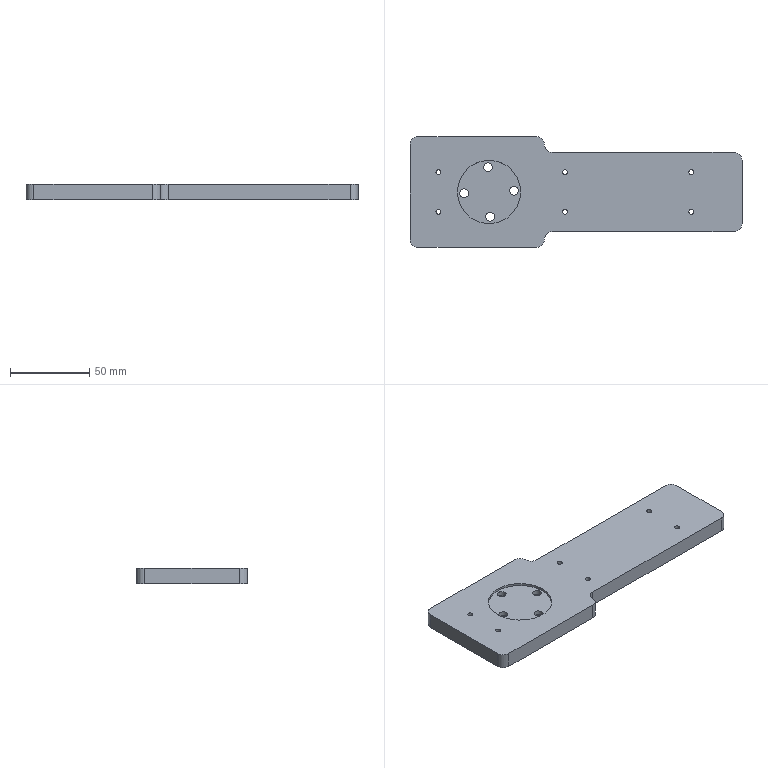Part | STEP file | SynoNew-0304-038 | 1 solid | 38 faces | box 210 x 70 x 10 mm | volume 117309 mm3 | cylinder 24 | plane 14 | commonest cylinder face diameters 10 x12 3.2 x6 5.5 x4 4 x1 40.02 x1
STEP:
#1=CARTESIAN_POINT('',(51.,0.,0.));
#2=VERTEX_POINT('',#1);
#3=CARTESIAN_POINT('',(55.,0.,0.));
#4=VERTEX_POINT('',#3);
#5=CARTESIAN_POINT('',(53.,0.,0.));
#6=DIRECTION('',(0.,0.,1.));
#7=DIRECTION('',(-1.,0.,0.));
#8=AXIS2_PLACEMENT_3D('',#5,#6,#7);
#9=CIRCLE('',#8,2.);
#10=EDGE_CURVE('',#2,#4,#9,.T.);
#11=ORIENTED_EDGE('',*,*,#10,.F.);
#12=CARTESIAN_POINT('',(53.,0.,0.));
#13=DIRECTION('',(0.,0.,1.));
#14=DIRECTION('',(-1.,0.,0.));
#15=AXIS2_PLACEMENT_3D('',#12,#13,#14);
#16=CIRCLE('',#15,2.);
#17=EDGE_CURVE('',#4,#2,#16,.T.);
#18=ORIENTED_EDGE('',*,*,#17,.F.);
#19=CARTESIAN_POINT('',(55.,0.,4.));
#20=VERTEX_POINT('',#19);
#21=CARTESIAN_POINT('',(55.,0.,0.));
#22=DIRECTION('',(0.,0.,1.));
#23=VECTOR('',#22,2.);
#24=LINE('',#21,#23);
#25=EDGE_CURVE('',#4,#20,#24,.T.);
#26=ORIENTED_EDGE('',*,*,#25,.T.);
#27=CARTESIAN_POINT('',(51.,0.,4.));
#28=VERTEX_POINT('',#27);
#29=CARTESIAN_POINT('',(53.,0.,4.));
#30=DIRECTION('',(0.,0.,1.));
#31=DIRECTION('',(-1.,0.,0.));
#32=AXIS2_PLACEMENT_3D('',#29,#30,#31);
#33=CIRCLE('',#32,2.);
#34=EDGE_CURVE('',#20,#28,#33,.T.);
#35=ORIENTED_EDGE('',*,*,#34,.T.);
#36=CARTESIAN_POINT('',(53.,0.,4.));
#37=DIRECTION('',(0.,0.,1.));
#38=DIRECTION('',(-1.,0.,0.));
#39=AXIS2_PLACEMENT_3D('',#36,#37,#38);
#40=CIRCLE('',#39,2.);
#41=EDGE_CURVE('',#28,#20,#40,.T.);
#42=ORIENTED_EDGE('',*,*,#41,.T.);
#43=ORIENTED_EDGE('',*,*,#25,.F.);
#44=EDGE_LOOP('',(#11,#18,#26,#35,#42,#43));
#45=FACE_OUTER_BOUND('',#44,.T.);
#46=CARTESIAN_POINT('',(53.,0.,0.));
#47=DIRECTION('',(0.,0.,1.));
#48=DIRECTION('',(-1.,0.,0.));
#49=AXIS2_PLACEMENT_3D('',#46,#47,#48);
#50=CYLINDRICAL_SURFACE('',#49,2.);
#51=ADVANCED_FACE('',(#45),#50,.F.);
#52=ORIENTED_EDGE('',*,*,#41,.F.);
#53=ORIENTED_EDGE('',*,*,#34,.F.);
#54=EDGE_LOOP('',(#52,#53));
#55=FACE_OUTER_BOUND('',#54,.T.);
#56=CARTESIAN_POINT('',(53.,0.,4.));
#57=DIRECTION('',(0.,0.,-1.));
#58=DIRECTION('',(-1.,0.,0.));
#59=AXIS2_PLACEMENT_3D('',#56,#57,#58);
#60=PLANE('',#59);
#61=ADVANCED_FACE('',(#55),#60,.T.);
#62=CARTESIAN_POINT('',(-105.4,-12.5,10.));
#63=VERTEX_POINT('',#62);
#64=CARTESIAN_POINT('',(-108.6,-12.5,10.));
#65=VERTEX_POINT('',#64);
#66=CARTESIAN_POINT('',(-107.,-12.5,10.));
#67=DIRECTION('',(0.,0.,-1.));
#68=DIRECTION('',(1.,0.,0.));
#69=AXIS2_PLACEMENT_3D('',#66,#67,#68);
#70=CIRCLE('',#69,1.6);
#71=EDGE_CURVE('',#63,#65,#70,.T.);
#72=ORIENTED_EDGE('',*,*,#71,.F.);
#73=CARTESIAN_POINT('',(-107.,-12.5,10.));
#74=DIRECTION('',(0.,0.,-1.));
#75=DIRECTION('',(1.,0.,0.));
#76=AXIS2_PLACEMENT_3D('',#73,#74,#75);
#77=CIRCLE('',#76,1.6);
#78=EDGE_CURVE('',#65,#63,#77,.T.);
#79=ORIENTED_EDGE('',*,*,#78,.F.);
#80=CARTESIAN_POINT('',(-108.6,-12.5,0.));
#81=VERTEX_POINT('',#80);
#82=CARTESIAN_POINT('',(-108.6,-12.5,-211.585));
#83=DIRECTION('',(0.,0.,-1.));
#84=VECTOR('',#83,1.6);
#85=LINE('',#82,#84);
#86=EDGE_CURVE('',#65,#81,#85,.T.);
#87=ORIENTED_EDGE('',*,*,#86,.T.);
#88=CARTESIAN_POINT('',(-107.,-12.5,0.));
#89=DIRECTION('',(0.,0.,1.));
#90=DIRECTION('',(1.,0.,0.));
#91=AXIS2_PLACEMENT_3D('',#88,#89,#90);
#92=CIRCLE('',#91,1.6);
#93=EDGE_CURVE('',#81,#81,#92,.T.);
#94=ORIENTED_EDGE('',*,*,#93,.F.);
#95=ORIENTED_EDGE('',*,*,#86,.F.);
#96=EDGE_LOOP('',(#72,#79,#87,#94,#95));
#97=FACE_OUTER_BOUND('',#96,.T.);
#98=CARTESIAN_POINT('',(-107.,-12.5,-211.585));
#99=DIRECTION('',(0.,0.,1.));
#100=DIRECTION('',(1.,0.,0.));
#101=AXIS2_PLACEMENT_3D('',#98,#99,#100);
#102=CYLINDRICAL_SURFACE('',#101,1.6);
#103=ADVANCED_FACE('',(#97),#102,.F.);
#104=CARTESIAN_POINT('',(-25.4,-12.5,10.));
#105=VERTEX_POINT('',#104);
#106=CARTESIAN_POINT('',(-28.6,-12.5,10.));
#107=VERTEX_POINT('',#106);
#108=CARTESIAN_POINT('',(-27.,-12.5,10.));
#109=DIRECTION('',(0.,0.,-1.));
#110=DIRECTION('',(1.,0.,0.));
#111=AXIS2_PLACEMENT_3D('',#108,#109,#110);
#112=CIRCLE('',#111,1.6);
#113=EDGE_CURVE('',#105,#107,#112,.T.);
#114=ORIENTED_EDGE('',*,*,#113,.F.);
#115=CARTESIAN_POINT('',(-27.,-12.5,10.));
#116=DIRECTION('',(0.,0.,-1.));
#117=DIRECTION('',(1.,0.,0.));
#118=AXIS2_PLACEMENT_3D('',#115,#116,#117);
#119=CIRCLE('',#118,1.6);
#120=EDGE_CURVE('',#107,#105,#119,.T.);
#121=ORIENTED_EDGE('',*,*,#120,.F.);
#122=CARTESIAN_POINT('',(-28.6,-12.5,0.));
#123=VERTEX_POINT('',#122);
#124=CARTESIAN_POINT('',(-28.6,-12.5,-211.585));
#125=DIRECTION('',(0.,0.,-1.));
#126=VECTOR('',#125,1.6);
#127=LINE('',#124,#126);
#128=EDGE_CURVE('',#107,#123,#127,.T.);
#129=ORIENTED_EDGE('',*,*,#128,.T.);
#130=CARTESIAN_POINT('',(-27.,-12.5,0.));
#131=DIRECTION('',(0.,0.,1.));
#132=DIRECTION('',(1.,0.,0.));
#133=AXIS2_PLACEMENT_3D('',#130,#131,#132);
#134=CIRCLE('',#133,1.6);
#135=EDGE_CURVE('',#123,#123,#134,.T.);
#136=ORIENTED_EDGE('',*,*,#135,.F.);
#137=ORIENTED_EDGE('',*,*,#128,.F.);
#138=EDGE_LOOP('',(#114,#121,#129,#136,#137));
#139=FACE_OUTER_BOUND('',#138,.T.);
#140=CARTESIAN_POINT('',(-27.,-12.5,-211.585));
#141=DIRECTION('',(0.,0.,1.));
#142=DIRECTION('',(1.,0.,0.));
#143=AXIS2_PLACEMENT_3D('',#140,#141,#142);
#144=CYLINDRICAL_SURFACE('',#143,1.6);
#145=ADVANCED_FACE('',(#139),#144,.F.);
#146=CARTESIAN_POINT('',(54.6,12.5,10.));
#147=VERTEX_POINT('',#146);
#148=CARTESIAN_POINT('',(51.4,12.5,10.));
#149=VERTEX_POINT('',#148);
#150=CARTESIAN_POINT('',(53.,12.5,10.));
#151=DIRECTION('',(0.,0.,-1.));
#152=DIRECTION('',(1.,0.,0.));
#153=AXIS2_PLACEMENT_3D('',#150,#151,#152);
#154=CIRCLE('',#153,1.6);
#155=EDGE_CURVE('',#147,#149,#154,.T.);
#156=ORIENTED_EDGE('',*,*,#155,.F.);
#157=CARTESIAN_POINT('',(53.,12.5,10.));
#158=DIRECTION('',(0.,0.,-1.));
#159=DIRECTION('',(1.,0.,0.));
#160=AXIS2_PLACEMENT_3D('',#157,#158,#159);
#161=CIRCLE('',#160,1.6);
#162=EDGE_CURVE('',#149,#147,#161,.T.);
#163=ORIENTED_EDGE('',*,*,#162,.F.);
#164=CARTESIAN_POINT('',(51.4,12.5,0.));
#165=VERTEX_POINT('',#164);
#166=CARTESIAN_POINT('',(51.4,12.5,-211.585));
#167=DIRECTION('',(0.,0.,-1.));
#168=VECTOR('',#167,1.6);
#169=LINE('',#166,#168);
#170=EDGE_CURVE('',#149,#165,#169,.T.);
#171=ORIENTED_EDGE('',*,*,#170,.T.);
#172=CARTESIAN_POINT('',(53.,12.5,0.));
#173=DIRECTION('',(0.,0.,1.));
#174=DIRECTION('',(1.,0.,0.));
#175=AXIS2_PLACEMENT_3D('',#172,#173,#174);
#176=CIRCLE('',#175,1.6);
#177=EDGE_CURVE('',#165,#165,#176,.T.);
#178=ORIENTED_EDGE('',*,*,#177,.F.);
#179=ORIENTED_EDGE('',*,*,#170,.F.);
#180=EDGE_LOOP('',(#156,#163,#171,#178,#179));
#181=FACE_OUTER_BOUND('',#180,.T.);
#182=CARTESIAN_POINT('',(53.,12.5,-211.585));
#183=DIRECTION('',(0.,0.,1.));
#184=DIRECTION('',(1.,0.,0.));
#185=AXIS2_PLACEMENT_3D('',#182,#183,#184);
#186=CYLINDRICAL_SURFACE('',#185,1.6);
#187=ADVANCED_FACE('',(#181),#186,.F.);
#188=CARTESIAN_POINT('',(54.6,-12.5,10.));
#189=VERTEX_POINT('',#188);
#190=CARTESIAN_POINT('',(51.4,-12.5,10.));
#191=VERTEX_POINT('',#190);
#192=CARTESIAN_POINT('',(53.,-12.5,10.));
#193=DIRECTION('',(0.,0.,-1.));
#194=DIRECTION('',(1.,0.,0.));
#195=AXIS2_PLACEMENT_3D('',#192,#193,#194);
#196=CIRCLE('',#195,1.6);
#197=EDGE_CURVE('',#189,#191,#196,.T.);
#198=ORIENTED_EDGE('',*,*,#197,.F.);
#199=CARTESIAN_POINT('',(53.,-12.5,10.));
#200=DIRECTION('',(0.,0.,-1.));
#201=DIRECTION('',(1.,0.,0.));
#202=AXIS2_PLACEMENT_3D('',#199,#200,#201);
#203=CIRCLE('',#202,1.6);
#204=EDGE_CURVE('',#191,#189,#203,.T.);
#205=ORIENTED_EDGE('',*,*,#204,.F.);
#206=CARTESIAN_POINT('',(51.4,-12.5,0.));
#207=VERTEX_POINT('',#206);
#208=CARTESIAN_POINT('',(51.4,-12.5,-211.585));
#209=DIRECTION('',(0.,0.,-1.));
#210=VECTOR('',#209,1.6);
#211=LINE('',#208,#210);
#212=EDGE_CURVE('',#191,#207,#211,.T.);
#213=ORIENTED_EDGE('',*,*,#212,.T.);
#214=CARTESIAN_POINT('',(53.,-12.5,0.));
#215=DIRECTION('',(0.,0.,1.));
#216=DIRECTION('',(1.,0.,0.));
#217=AXIS2_PLACEMENT_3D('',#214,#215,#216);
#218=CIRCLE('',#217,1.6);
#219=EDGE_CURVE('',#207,#207,#218,.T.);
#220=ORIENTED_EDGE('',*,*,#219,.F.);
#221=ORIENTED_EDGE('',*,*,#212,.F.);
#222=EDGE_LOOP('',(#198,#205,#213,#220,#221));
#223=FACE_OUTER_BOUND('',#222,.T.);
#224=CARTESIAN_POINT('',(53.,-12.5,-211.585));
#225=DIRECTION('',(0.,0.,1.));
#226=DIRECTION('',(1.,0.,0.));
#227=AXIS2_PLACEMENT_3D('',#224,#225,#226);
#228=CYLINDRICAL_SURFACE('',#227,1.6);
#229=ADVANCED_FACE('',(#223),#228,.F.);
#230=CARTESIAN_POINT('',(-25.4,12.5,10.));
#231=VERTEX_POINT('',#230);
#232=CARTESIAN_POINT('',(-28.6,12.5,10.));
#233=VERTEX_POINT('',#232);
#234=CARTESIAN_POINT('',(-27.,12.5,10.));
#235=DIRECTION('',(0.,0.,-1.));
#236=DIRECTION('',(1.,0.,0.));
#237=AXIS2_PLACEMENT_3D('',#234,#235,#236);
#238=CIRCLE('',#237,1.6);
#239=EDGE_CURVE('',#231,#233,#238,.T.);
#240=ORIENTED_EDGE('',*,*,#239,.F.);
#241=CARTESIAN_POINT('',(-27.,12.5,10.));
#242=DIRECTION('',(0.,0.,-1.));
#243=DIRECTION('',(1.,0.,0.));
#244=AXIS2_PLACEMENT_3D('',#241,#242,#243);
#245=CIRCLE('',#244,1.6);
#246=EDGE_CURVE('',#233,#231,#245,.T.);
#247=ORIENTED_EDGE('',*,*,#246,.F.);
#248=CARTESIAN_POINT('',(-28.6,12.5,0.));
#249=VERTEX_POINT('',#248);
#250=CARTESIAN_POINT('',(-28.6,12.5,-211.585));
#251=DIRECTION('',(0.,0.,-1.));
#252=VECTOR('',#251,1.6);
#253=LINE('',#250,#252);
#254=EDGE_CURVE('',#233,#249,#253,.T.);
#255=ORIENTED_EDGE('',*,*,#254,.T.);
#256=CARTESIAN_POINT('',(-27.,12.5,0.));
#257=DIRECTION('',(0.,0.,1.));
#258=DIRECTION('',(1.,0.,0.));
#259=AXIS2_PLACEMENT_3D('',#256,#257,#258);
#260=CIRCLE('',#259,1.6);
#261=EDGE_CURVE('',#249,#249,#260,.T.);
#262=ORIENTED_EDGE('',*,*,#261,.F.);
#263=ORIENTED_EDGE('',*,*,#254,.F.);
#264=EDGE_LOOP('',(#240,#247,#255,#262,#263));
#265=FACE_OUTER_BOUND('',#264,.T.);
#266=CARTESIAN_POINT('',(-27.,12.5,-211.585));
#267=DIRECTION('',(0.,0.,1.));
#268=DIRECTION('',(1.,0.,0.));
#269=AXIS2_PLACEMENT_3D('',#266,#267,#268);
#270=CYLINDRICAL_SURFACE('',#269,1.6);
#271=ADVANCED_FACE('',(#265),#270,.F.);
#272=CARTESIAN_POINT('',(-105.4,12.5,10.));
#273=VERTEX_POINT('',#272);
#274=CARTESIAN_POINT('',(-108.6,12.5,10.));
#275=VERTEX_POINT('',#274);
#276=CARTESIAN_POINT('',(-107.,12.5,10.));
#277=DIRECTION('',(0.,0.,-1.));
#278=DIRECTION('',(1.,0.,0.));
#279=AXIS2_PLACEMENT_3D('',#276,#277,#278);
#280=CIRCLE('',#279,1.6);
#281=EDGE_CURVE('',#273,#275,#280,.T.);
#282=ORIENTED_EDGE('',*,*,#281,.F.);
#283=CARTESIAN_POINT('',(-107.,12.5,10.));
#284=DIRECTION('',(0.,0.,-1.));
#285=DIRECTION('',(1.,0.,0.));
#286=AXIS2_PLACEMENT_3D('',#283,#284,#285);
#287=CIRCLE('',#286,1.6);
#288=EDGE_CURVE('',#275,#273,#287,.T.);
#289=ORIENTED_EDGE('',*,*,#288,.F.);
#290=CARTESIAN_POINT('',(-108.6,12.5,0.));
#291=VERTEX_POINT('',#290);
#292=CARTESIAN_POINT('',(-108.6,12.5,-211.585));
#293=DIRECTION('',(0.,0.,-1.));
#294=VECTOR('',#293,1.6);
#295=LINE('',#292,#294);
#296=EDGE_CURVE('',#275,#291,#295,.T.);
#297=ORIENTED_EDGE('',*,*,#296,.T.);
#298=CARTESIAN_POINT('',(-107.,12.5,0.));
#299=DIRECTION('',(0.,0.,1.));
#300=DIRECTION('',(1.,0.,0.));
#301=AXIS2_PLACEMENT_3D('',#298,#299,#300);
#302=CIRCLE('',#301,1.6);
#303=EDGE_CURVE('',#291,#291,#302,.T.);
#304=ORIENTED_EDGE('',*,*,#303,.F.);
#305=ORIENTED_EDGE('',*,*,#296,.F.);
#306=EDGE_LOOP('',(#282,#289,#297,#304,#305));
#307=FACE_OUTER_BOUND('',#306,.T.);
#308=CARTESIAN_POINT('',(-107.,12.5,-211.585));
#309=DIRECTION('',(0.,0.,1.));
#310=DIRECTION('',(1.,0.,0.));
#311=AXIS2_PLACEMENT_3D('',#308,#309,#310);
#312=CYLINDRICAL_SURFACE('',#311,1.6);
#313=ADVANCED_FACE('',(#307),#312,.F.);
#314=CARTESIAN_POINT('',(85.,-20.,10.));
#315=VERTEX_POINT('',#314);
#316=CARTESIAN_POINT('',(80.,-25.,10.));
#317=VERTEX_POINT('',#316);
#318=CARTESIAN_POINT('',(80.,-20.,10.));
#319=DIRECTION('',(0.,0.,-1.));
#320=DIRECTION('',(0.7071,-0.7071,0.));
#321=AXIS2_PLACEMENT_3D('',#318,#319,#320);
#322=CIRCLE('',#321,5.);
#323=EDGE_CURVE('',#315,#317,#322,.T.);
#324=ORIENTED_EDGE('',*,*,#323,.T.);
#325=CARTESIAN_POINT('',(80.,-25.,0.));
#326=VERTEX_POINT('',#325);
#327=CARTESIAN_POINT('',(80.,-25.,5.));
#328=DIRECTION('',(0.,0.,-1.));
#329=VECTOR('',#328,10.);
#330=LINE('',#327,#329);
#331=EDGE_CURVE('',#317,#326,#330,.T.);
#332=ORIENTED_EDGE('',*,*,#331,.T.);
#333=CARTESIAN_POINT('',(85.,-20.,0.));
#334=VERTEX_POINT('',#333);
#335=CARTESIAN_POINT('',(80.,-20.,0.));
#336=DIRECTION('',(0.,0.,1.));
#337=DIRECTION('',(0.7071,-0.7071,0.));
#338=AXIS2_PLACEMENT_3D('',#335,#336,#337);
#339=CIRCLE('',#338,5.);
#340=EDGE_CURVE('',#326,#334,#339,.T.);
#341=ORIENTED_EDGE('',*,*,#340,.T.);
#342=CARTESIAN_POINT('',(85.,-20.,5.));
#343=DIRECTION('',(0.,0.,1.));
#344=VECTOR('',#343,10.);
#345=LINE('',#342,#344);
#346=EDGE_CURVE('',#334,#315,#345,.T.);
#347=ORIENTED_EDGE('',*,*,#346,.T.);
#348=EDGE_LOOP('',(#324,#332,#341,#347));
#349=FACE_OUTER_BOUND('',#348,.T.);
#350=CARTESIAN_POINT('',(80.,-20.,5.));
#351=DIRECTION('',(0.,0.,1.));
#352=DIRECTION('',(0.7071,-0.7071,0.));
#353=AXIS2_PLACEMENT_3D('',#350,#351,#352);
#354=CYLINDRICAL_SURFACE('',#353,5.);
#355=ADVANCED_FACE('',(#349),#354,.T.);
#356=ORIENTED_EDGE('',*,*,#346,.F.);
#357=CARTESIAN_POINT('',(85.,20.,0.));
#358=VERTEX_POINT('',#357);
#359=CARTESIAN_POINT('',(85.,-20.043,0.));
#360=DIRECTION('',(0.,-1.,0.));
#361=VECTOR('',#360,10.);
#362=LINE('',#359,#361);
#363=EDGE_CURVE('',#358,#334,#362,.T.);
#364=ORIENTED_EDGE('',*,*,#363,.F.);
#365=CARTESIAN_POINT('',(85.,20.,10.));
#366=VERTEX_POINT('',#365);
#367=CARTESIAN_POINT('',(85.,20.,5.));
#368=DIRECTION('',(0.,0.,-1.));
#369=VECTOR('',#368,10.);
#370=LINE('',#367,#369);
#371=EDGE_CURVE('',#366,#358,#370,.T.);
#372=ORIENTED_EDGE('',*,*,#371,.F.);
#373=CARTESIAN_POINT('',(85.,-20.043,10.));
#374=DIRECTION('',(0.,1.,0.));
#375=VECTOR('',#374,10.);
#376=LINE('',#373,#375);
#377=EDGE_CURVE('',#315,#366,#376,.T.);
#378=ORIENTED_EDGE('',*,*,#377,.F.);
#379=EDGE_LOOP('',(#356,#364,#372,#378));
#380=FACE_OUTER_BOUND('',#379,.T.);
#381=CARTESIAN_POINT('',(85.,-40.087,10.));
#382=DIRECTION('',(-1.,0.,0.));
#383=DIRECTION('',(0.,1.,0.));
#384=AXIS2_PLACEMENT_3D('',#381,#382,#383);
#385=PLANE('',#384);
#386=ADVANCED_FACE('',(#380),#385,.F.);
#387=ORIENTED_EDGE('',*,*,#340,.F.);
#388=CARTESIAN_POINT('',(-35.,-25.,0.));
#389=VERTEX_POINT('',#388);
#390=CARTESIAN_POINT('',(70.95,-25.,0.));
#391=DIRECTION('',(-1.,0.,0.));
#392=VECTOR('',#391,10.);
#393=LINE('',#390,#392);
#394=EDGE_CURVE('',#326,#389,#393,.T.);
#395=ORIENTED_EDGE('',*,*,#394,.T.);
#396=CARTESIAN_POINT('',(-40.,-30.,0.));
#397=VERTEX_POINT('',#396);
#398=CARTESIAN_POINT('',(-35.,-30.,0.));
#399=DIRECTION('',(0.,0.,-1.));
#400=DIRECTION('',(-0.7071,0.7071,0.));
#401=AXIS2_PLACEMENT_3D('',#398,#399,#400);
#402=CIRCLE('',#401,5.);
#403=EDGE_CURVE('',#397,#389,#402,.T.);
#404=ORIENTED_EDGE('',*,*,#403,.F.);
#405=CARTESIAN_POINT('',(-45.,-35.,0.));
#406=VERTEX_POINT('',#405);
#407=CARTESIAN_POINT('',(-45.,-30.,0.));
#408=DIRECTION('',(0.,0.,1.));
#409=DIRECTION('',(0.7071,-0.7071,0.));
#410=AXIS2_PLACEMENT_3D('',#407,#408,#409);
#411=CIRCLE('',#410,5.);
#412=EDGE_CURVE('',#406,#397,#411,.T.);
#413=ORIENTED_EDGE('',*,*,#412,.F.);
#414=CARTESIAN_POINT('',(-120.,-35.,0.));
#415=VERTEX_POINT('',#414);
#416=CARTESIAN_POINT('',(-125.,-35.,0.));
#417=DIRECTION('',(1.,0.,0.));
#418=VECTOR('',#417,10.);
#419=LINE('',#416,#418);
#420=EDGE_CURVE('',#415,#406,#419,.T.);
#421=ORIENTED_EDGE('',*,*,#420,.F.);
#422=CARTESIAN_POINT('',(-125.,-30.,0.));
#423=VERTEX_POINT('',#422);
#424=CARTESIAN_POINT('',(-120.,-30.,0.));
#425=DIRECTION('',(0.,0.,1.));
#426=DIRECTION('',(-0.7071,-0.7071,0.));
#427=AXIS2_PLACEMENT_3D('',#424,#425,#426);
#428=CIRCLE('',#427,5.);
#429=EDGE_CURVE('',#423,#415,#428,.T.);
#430=ORIENTED_EDGE('',*,*,#429,.F.);
#431=CARTESIAN_POINT('',(-125.,30.,0.));
#432=VERTEX_POINT('',#431);
#433=CARTESIAN_POINT('',(-125.,35.,0.));
#434=DIRECTION('',(0.,-1.,0.));
#435=VECTOR('',#434,10.);
#436=LINE('',#433,#435);
#437=EDGE_CURVE('',#432,#423,#436,.T.);
#438=ORIENTED_EDGE('',*,*,#437,.F.);
#439=CARTESIAN_POINT('',(-120.,35.,0.));
#440=VERTEX_POINT('',#439);
#441=CARTESIAN_POINT('',(-120.,30.,0.));
#442=DIRECTION('',(0.,0.,1.));
#443=DIRECTION('',(-0.7071,0.7071,0.));
#444=AXIS2_PLACEMENT_3D('',#441,#442,#443);
#445=CIRCLE('',#444,5.);
#446=EDGE_CURVE('',#440,#432,#445,.T.);
#447=ORIENTED_EDGE('',*,*,#446,.F.);
#448=CARTESIAN_POINT('',(-45.,35.,0.));
#449=VERTEX_POINT('',#448);
#450=CARTESIAN_POINT('',(125.,35.,0.));
#451=DIRECTION('',(-1.,0.,0.));
#452=VECTOR('',#451,10.);
#453=LINE('',#450,#452);
#454=EDGE_CURVE('',#449,#440,#453,.T.);
#455=ORIENTED_EDGE('',*,*,#454,.F.);
#456=CARTESIAN_POINT('',(-40.,30.,0.));
#457=VERTEX_POINT('',#456);
#458=CARTESIAN_POINT('',(-45.,30.,0.));
#459=DIRECTION('',(0.,0.,1.));
#460=DIRECTION('',(0.7071,0.7071,0.));
#461=AXIS2_PLACEMENT_3D('',#458,#459,#460);
#462=CIRCLE('',#461,5.);
#463=EDGE_CURVE('',#457,#449,#462,.T.);
#464=ORIENTED_EDGE('',*,*,#463,.F.);
#465=CARTESIAN_POINT('',(-35.,25.,0.));
#466=VERTEX_POINT('',#465);
#467=CARTESIAN_POINT('',(-35.,30.,0.));
#468=DIRECTION('',(0.,0.,-1.));
#469=DIRECTION('',(-0.7071,-0.7071,0.));
#470=AXIS2_PLACEMENT_3D('',#467,#468,#469);
#471=CIRCLE('',#470,5.);
#472=EDGE_CURVE('',#466,#457,#471,.T.);
#473=ORIENTED_EDGE('',*,*,#472,.F.);
#474=CARTESIAN_POINT('',(80.,25.,0.));
#475=VERTEX_POINT('',#474);
#476=CARTESIAN_POINT('',(-20.,25.,0.));
#477=DIRECTION('',(1.,0.,0.));
#478=VECTOR('',#477,10.);
#479=LINE('',#476,#478);
#480=EDGE_CURVE('',#466,#475,#479,.T.);
#481=ORIENTED_EDGE('',*,*,#480,.T.);
#482=CARTESIAN_POINT('',(80.,20.,0.));
#483=DIRECTION('',(0.,0.,1.));
#484=DIRECTION('',(0.7071,0.7071,0.));
#485=AXIS2_PLACEMENT_3D('',#482,#483,#484);
#486=CIRCLE('',#485,5.);
#487=EDGE_CURVE('',#358,#475,#486,.T.);
#488=ORIENTED_EDGE('',*,*,#487,.F.);
#489=ORIENTED_EDGE('',*,*,#363,.T.);
#490=EDGE_LOOP('',(#387,#395,#404,#413,#421,#430,#438,#447,#455,#464,#473,#481,#488,#489));
#491=FACE_OUTER_BOUND('',#490,.T.);
#492=ORIENTED_EDGE('',*,*,#10,.T.);
#493=ORIENTED_EDGE('',*,*,#17,.T.);
#494=EDGE_LOOP('',(#492,#493));
#495=FACE_BOUND('',#494,.T.);
#496=ORIENTED_EDGE('',*,*,#93,.T.);
#497=EDGE_LOOP('',(#496));
#498=FACE_BOUND('',#497,.T.);
#499=ORIENTED_EDGE('',*,*,#135,.T.);
#500=EDGE_LOOP('',(#499));
#501=FACE_BOUND('',#500,.T.);
#502=ORIENTED_EDGE('',*,*,#177,.T.);
#503=EDGE_LOOP('',(#502));
#504=FACE_BOUND('',#503,.T.);
#505=ORIENTED_EDGE('',*,*,#219,.T.);
#506=EDGE_LOOP('',(#505));
#507=FACE_BOUND('',#506,.T.);
#508=ORIENTED_EDGE('',*,*,#261,.T.);
#509=EDGE_LOOP('',(#508));
#510=FACE_BOUND('',#509,.T.);
#511=ORIENTED_EDGE('',*,*,#303,.T.);
#512=EDGE_LOOP('',(#511));
#513=FACE_BOUND('',#512,.T.);
#514=CARTESIAN_POINT('',(-79.276,-15.733,0.));
#515=VERTEX_POINT('',#514);
#516=CARTESIAN_POINT('',(-69.276,-15.733,0.));
#517=VERTEX_POINT('',#516);
#518=CARTESIAN_POINT('',(-74.276,-15.733,0.));
#519=DIRECTION('',(0.,0.,1.));
#520=DIRECTION('',(-1.,0.,0.));
#521=AXIS2_PLACEMENT_3D('',#518,#519,#520);
#522=CIRCLE('',#521,5.);
#523=EDGE_CURVE('',#515,#517,#522,.T.);
#524=ORIENTED_EDGE('',*,*,#523,.T.);
#525=CARTESIAN_POINT('',(-74.276,-15.733,0.));
#526=DIRECTION('',(0.,0.,1.));
#527=DIRECTION('',(-1.,0.,0.));
#528=AXIS2_PLACEMENT_3D('',#525,#526,#527);
#529=CIRCLE('',#528,5.);
#530=EDGE_CURVE('',#517,#515,#529,.T.);
#531=ORIENTED_EDGE('',*,*,#530,.T.);
#532=EDGE_LOOP('',(#524,#531));
#533=FACE_BOUND('',#532,.T.);
#534=CARTESIAN_POINT('',(-64.267,0.7236,0.));
#535=VERTEX_POINT('',#534);
#536=CARTESIAN_POINT('',(-54.267,0.7236,0.));
#537=VERTEX_POINT('',#536);
#538=CARTESIAN_POINT('',(-59.267,0.7236,0.));
#539=DIRECTION('',(0.,0.,1.));
#540=DIRECTION('',(-1.,0.,0.));
#541=AXIS2_PLACEMENT_3D('',#538,#539,#540);
#542=CIRCLE('',#541,5.);
#543=EDGE_CURVE('',#535,#537,#542,.T.);
#544=ORIENTED_EDGE('',*,*,#543,.T.);
#545=CARTESIAN_POINT('',(-59.267,0.7236,0.));
#546=DIRECTION('',(0.,0.,1.));
#547=DIRECTION('',(-1.,0.,0.));
#548=AXIS2_PLACEMENT_3D('',#545,#546,#547);
#549=CIRCLE('',#548,5.);
#550=EDGE_CURVE('',#537,#535,#549,.T.);
#551=ORIENTED_EDGE('',*,*,#550,.T.);
#552=EDGE_LOOP('',(#544,#551));
#553=FACE_BOUND('',#552,.T.);
#554=CARTESIAN_POINT('',(-80.724,15.733,0.));
#555=VERTEX_POINT('',#554);
#556=CARTESIAN_POINT('',(-70.724,15.733,0.));
#557=VERTEX_POINT('',#556);
#558=CARTESIAN_POINT('',(-75.724,15.733,0.));
#559=DIRECTION('',(0.,0.,1.));
#560=DIRECTION('',(-1.,0.,0.));
#561=AXIS2_PLACEMENT_3D('',#558,#559,#560);
#562=CIRCLE('',#561,5.);
#563=EDGE_CURVE('',#555,#557,#562,.T.);
#564=ORIENTED_EDGE('',*,*,#563,.T.);
#565=CARTESIAN_POINT('',(-75.724,15.733,0.));
#566=DIRECTION('',(0.,0.,1.));
#567=DIRECTION('',(-1.,0.,0.));
#568=AXIS2_PLACEMENT_3D('',#565,#566,#567);
#569=CIRCLE('',#568,5.);
#570=EDGE_CURVE('',#557,#555,#569,.T.);
#571=ORIENTED_EDGE('',*,*,#570,.T.);
#572=EDGE_LOOP('',(#564,#571));
#573=FACE_BOUND('',#572,.T.);
#574=CARTESIAN_POINT('',(-95.733,-0.7236,0.));
#575=VERTEX_POINT('',#574);
#576=CARTESIAN_POINT('',(-85.733,-0.7236,0.));
#577=VERTEX_POINT('',#576);
#578=CARTESIAN_POINT('',(-90.733,-0.7236,0.));
#579=DIRECTION('',(0.,0.,1.));
#580=DIRECTION('',(-1.,0.,0.));
#581=AXIS2_PLACEMENT_3D('',#578,#579,#580);
#582=CIRCLE('',#581,5.);
#583=EDGE_CURVE('',#575,#577,#582,.T.);
#584=ORIENTED_EDGE('',*,*,#583,.T.);
#585=CARTESIAN_POINT('',(-90.733,-0.7236,0.));
#586=DIRECTION('',(0.,0.,1.));
#587=DIRECTION('',(-1.,0.,0.));
#588=AXIS2_PLACEMENT_3D('',#585,#586,#587);
#589=CIRCLE('',#588,5.);
#590=EDGE_CURVE('',#577,#575,#589,.T.);
#591=ORIENTED_EDGE('',*,*,#590,.T.);
#592=EDGE_LOOP('',(#584,#591));
#593=FACE_BOUND('',#592,.T.);
#594=CARTESIAN_POINT('',(0.,0.,0.));
#595=DIRECTION('',(0.,0.,1.));
#596=DIRECTION('',(1.,0.,0.));
#597=AXIS2_PLACEMENT_3D('',#594,#595,#596);
#598=PLANE('',#597);
#599=ADVANCED_FACE('',(#491,#495,#498,#501,#504,#507,#510,#513,#533,#553,#573,#593),#598,.F.);
#600=ORIENTED_EDGE('',*,*,#487,.T.);
#601=CARTESIAN_POINT('',(80.,25.,10.));
#602=VERTEX_POINT('',#601);
#603=CARTESIAN_POINT('',(80.,25.,5.));
#604=DIRECTION('',(0.,0.,1.));
#605=VECTOR('',#604,10.);
#606=LINE('',#603,#605);
#607=EDGE_CURVE('',#475,#602,#606,.T.);
#608=ORIENTED_EDGE('',*,*,#607,.T.);
#609=CARTESIAN_POINT('',(80.,20.,10.));
#610=DIRECTION('',(0.,0.,-1.));
#611=DIRECTION('',(0.7071,0.7071,0.));
#612=AXIS2_PLACEMENT_3D('',#609,#610,#611);
#613=CIRCLE('',#612,5.);
#614=EDGE_CURVE('',#602,#366,#613,.T.);
#615=ORIENTED_EDGE('',*,*,#614,.T.);
#616=ORIENTED_EDGE('',*,*,#371,.T.);
#617=EDGE_LOOP('',(#600,#608,#615,#616));
#618=FACE_OUTER_BOUND('',#617,.T.);
#619=CARTESIAN_POINT('',(80.,20.,5.));
#620=DIRECTION('',(0.,0.,-1.));
#621=DIRECTION('',(0.7071,0.7071,0.));
#622=AXIS2_PLACEMENT_3D('',#619,#620,#621);
#623=CYLINDRICAL_SURFACE('',#622,5.);
#624=ADVANCED_FACE('',(#618),#623,.T.);
#625=ORIENTED_EDGE('',*,*,#331,.F.);
#626=CARTESIAN_POINT('',(-35.,-25.,10.));
#627=VERTEX_POINT('',#626);
#628=CARTESIAN_POINT('',(70.95,-25.,10.));
#629=DIRECTION('',(1.,0.,0.));
#630=VECTOR('',#629,10.);
#631=LINE('',#628,#630);
#632=EDGE_CURVE('',#627,#317,#631,.T.);
#633=ORIENTED_EDGE('',*,*,#632,.F.);
#634=CARTESIAN_POINT('',(-35.,-25.,0.));
#635=DIRECTION('',(0.,0.,1.));
#636=VECTOR('',#635,10.);
#637=LINE('',#634,#636);
#638=EDGE_CURVE('',#389,#627,#637,.T.);
#639=ORIENTED_EDGE('',*,*,#638,.F.);
#640=ORIENTED_EDGE('',*,*,#394,.F.);
#641=EDGE_LOOP('',(#625,#633,#639,#640));
#642=FACE_OUTER_BOUND('',#641,.T.);
#643=CARTESIAN_POINT('',(141.901,-25.,0.));
#644=DIRECTION('',(0.,1.,0.));
#645=DIRECTION('',(-1.,0.,0.));
#646=AXIS2_PLACEMENT_3D('',#643,#644,#645);
#647=PLANE('',#646);
#648=ADVANCED_FACE('',(#642),#647,.F.);
#649=ORIENTED_EDGE('',*,*,#323,.F.);
#650=ORIENTED_EDGE('',*,*,#377,.T.);
#651=ORIENTED_EDGE('',*,*,#614,.F.);
#652=CARTESIAN_POINT('',(-35.,25.,10.));
#653=VERTEX_POINT('',#652);
#654=CARTESIAN_POINT('',(-20.,25.,10.));
#655=DIRECTION('',(-1.,0.,0.));
#656=VECTOR('',#655,10.);
#657=LINE('',#654,#656);
#658=EDGE_CURVE('',#602,#653,#657,.T.);
#659=ORIENTED_EDGE('',*,*,#658,.T.);
#660=CARTESIAN_POINT('',(-40.,30.,10.));
#661=VERTEX_POINT('',#660);
#662=CARTESIAN_POINT('',(-35.,30.,10.));
#663=DIRECTION('',(0.,0.,1.));
#664=DIRECTION('',(-0.7071,-0.7071,0.));
#665=AXIS2_PLACEMENT_3D('',#662,#663,#664);
#666=CIRCLE('',#665,5.);
#667=EDGE_CURVE('',#661,#653,#666,.T.);
#668=ORIENTED_EDGE('',*,*,#667,.F.);
#669=CARTESIAN_POINT('',(-45.,35.,10.));
#670=VERTEX_POINT('',#669);
#671=CARTESIAN_POINT('',(-45.,30.,10.));
#672=DIRECTION('',(0.,0.,-1.));
#673=DIRECTION('',(0.7071,0.7071,0.));
#674=AXIS2_PLACEMENT_3D('',#671,#672,#673);
#675=CIRCLE('',#674,5.);
#676=EDGE_CURVE('',#670,#661,#675,.T.);
#677=ORIENTED_EDGE('',*,*,#676,.F.);
#678=CARTESIAN_POINT('',(-120.,35.,10.));
#679=VERTEX_POINT('',#678);
#680=CARTESIAN_POINT('',(125.,35.,10.));
#681=DIRECTION('',(-1.,0.,0.));
#682=VECTOR('',#681,10.);
#683=LINE('',#680,#682);
#684=EDGE_CURVE('',#670,#679,#683,.T.);
#685=ORIENTED_EDGE('',*,*,#684,.T.);
#686=CARTESIAN_POINT('',(-125.,30.,10.));
#687=VERTEX_POINT('',#686);
#688=CARTESIAN_POINT('',(-120.,30.,10.));
#689=DIRECTION('',(0.,0.,-1.));
#690=DIRECTION('',(-0.7071,0.7071,0.));
#691=AXIS2_PLACEMENT_3D('',#688,#689,#690);
#692=CIRCLE('',#691,5.);
#693=EDGE_CURVE('',#687,#679,#692,.T.);
#694=ORIENTED_EDGE('',*,*,#693,.F.);
#695=CARTESIAN_POINT('',(-125.,-30.,10.));
#696=VERTEX_POINT('',#695);
#697=CARTESIAN_POINT('',(-125.,35.,10.));
#698=DIRECTION('',(0.,-1.,0.));
#699=VECTOR('',#698,10.);
#700=LINE('',#697,#699);
#701=EDGE_CURVE('',#687,#696,#700,.T.);
#702=ORIENTED_EDGE('',*,*,#701,.T.);
#703=CARTESIAN_POINT('',(-120.,-35.,10.));
#704=VERTEX_POINT('',#703);
#705=CARTESIAN_POINT('',(-120.,-30.,10.));
#706=DIRECTION('',(0.,0.,-1.));
#707=DIRECTION('',(-0.7071,-0.7071,0.));
#708=AXIS2_PLACEMENT_3D('',#705,#706,#707);
#709=CIRCLE('',#708,5.);
#710=EDGE_CURVE('',#704,#696,#709,.T.);
#711=ORIENTED_EDGE('',*,*,#710,.F.);
#712=CARTESIAN_POINT('',(-45.,-35.,10.));
#713=VERTEX_POINT('',#712);
#714=CARTESIAN_POINT('',(-125.,-35.,10.));
#715=DIRECTION('',(1.,0.,0.));
#716=VECTOR('',#715,10.);
#717=LINE('',#714,#716);
#718=EDGE_CURVE('',#704,#713,#717,.T.);
#719=ORIENTED_EDGE('',*,*,#718,.T.);
#720=CARTESIAN_POINT('',(-40.,-30.,10.));
#721=VERTEX_POINT('',#720);
#722=CARTESIAN_POINT('',(-45.,-30.,10.));
#723=DIRECTION('',(0.,0.,-1.));
#724=DIRECTION('',(0.7071,-0.7071,0.));
#725=AXIS2_PLACEMENT_3D('',#722,#723,#724);
#726=CIRCLE('',#725,5.);
#727=EDGE_CURVE('',#721,#713,#726,.T.);
#728=ORIENTED_EDGE('',*,*,#727,.F.);
#729=CARTESIAN_POINT('',(-35.,-30.,10.));
#730=DIRECTION('',(0.,0.,1.));
#731=DIRECTION('',(-0.7071,0.7071,0.));
#732=AXIS2_PLACEMENT_3D('',#729,#730,#731);
#733=CIRCLE('',#732,5.);
#734=EDGE_CURVE('',#627,#721,#733,.T.);
#735=ORIENTED_EDGE('',*,*,#734,.F.);
#736=ORIENTED_EDGE('',*,*,#632,.T.);
#737=EDGE_LOOP('',(#649,#650,#651,#659,#668,#677,#685,#694,#702,#711,#719,#728,#735,#736));
#738=FACE_OUTER_BOUND('',#737,.T.);
#739=ORIENTED_EDGE('',*,*,#71,.T.);
#740=ORIENTED_EDGE('',*,*,#78,.T.);
#741=EDGE_LOOP('',(#739,#740));
#742=FACE_BOUND('',#741,.T.);
#743=ORIENTED_EDGE('',*,*,#113,.T.);
#744=ORIENTED_EDGE('',*,*,#120,.T.);
#745=EDGE_LOOP('',(#743,#744));
#746=FACE_BOUND('',#745,.T.);
#747=ORIENTED_EDGE('',*,*,#155,.T.);
#748=ORIENTED_EDGE('',*,*,#162,.T.);
#749=EDGE_LOOP('',(#747,#748));
#750=FACE_BOUND('',#749,.T.);
#751=ORIENTED_EDGE('',*,*,#197,.T.);
#752=ORIENTED_EDGE('',*,*,#204,.T.);
#753=EDGE_LOOP('',(#751,#752));
#754=FACE_BOUND('',#753,.T.);
#755=ORIENTED_EDGE('',*,*,#239,.T.);
#756=ORIENTED_EDGE('',*,*,#246,.T.);
#757=EDGE_LOOP('',(#755,#756));
#758=FACE_BOUND('',#757,.T.);
#759=ORIENTED_EDGE('',*,*,#281,.T.);
#760=ORIENTED_EDGE('',*,*,#288,.T.);
#761=EDGE_LOOP('',(#759,#760));
#762=FACE_BOUND('',#761,.T.);
#763=CARTESIAN_POINT('',(-54.99,0.,10.));
#764=VERTEX_POINT('',#763);
#765=CARTESIAN_POINT('',(-95.01,0.,10.));
#766=VERTEX_POINT('',#765);
#767=CARTESIAN_POINT('',(-75.,0.,10.));
#768=DIRECTION('',(0.,0.,-1.));
#769=DIRECTION('',(1.,0.,0.));
#770=AXIS2_PLACEMENT_3D('',#767,#768,#769);
#771=CIRCLE('',#770,20.01);
#772=EDGE_CURVE('',#764,#766,#771,.T.);
#773=ORIENTED_EDGE('',*,*,#772,.T.);
#774=CARTESIAN_POINT('',(-75.,0.,10.));
#775=DIRECTION('',(0.,0.,-1.));
#776=DIRECTION('',(1.,0.,0.));
#777=AXIS2_PLACEMENT_3D('',#774,#775,#776);
#778=CIRCLE('',#777,20.01);
#779=EDGE_CURVE('',#766,#764,#778,.T.);
#780=ORIENTED_EDGE('',*,*,#779,.T.);
#781=EDGE_LOOP('',(#773,#780));
#782=FACE_BOUND('',#781,.T.);
#783=CARTESIAN_POINT('',(0.,0.,10.));
#784=DIRECTION('',(0.,0.,1.));
#785=DIRECTION('',(1.,0.,0.));
#786=AXIS2_PLACEMENT_3D('',#783,#784,#785);
#787=PLANE('',#786);
#788=ADVANCED_FACE('',(#738,#742,#746,#750,#754,#758,#762,#782),#787,.T.);
#789=ORIENTED_EDGE('',*,*,#693,.T.);
#790=CARTESIAN_POINT('',(-120.,35.,0.));
#791=DIRECTION('',(0.,0.,-1.));
#792=VECTOR('',#791,10.);
#793=LINE('',#790,#792);
#794=EDGE_CURVE('',#679,#440,#793,.T.);
#795=ORIENTED_EDGE('',*,*,#794,.T.);
#796=ORIENTED_EDGE('',*,*,#446,.T.);
#797=CARTESIAN_POINT('',(-125.,30.,0.));
#798=DIRECTION('',(0.,0.,1.));
#799=VECTOR('',#798,10.);
#800=LINE('',#797,#799);
#801=EDGE_CURVE('',#432,#687,#800,.T.);
#802=ORIENTED_EDGE('',*,*,#801,.T.);
#803=EDGE_LOOP('',(#789,#795,#796,#802));
#804=FACE_OUTER_BOUND('',#803,.T.);
#805=CARTESIAN_POINT('',(-120.,30.,0.));
#806=DIRECTION('',(0.,0.,1.));
#807=DIRECTION('',(-0.7071,0.7071,0.));
#808=AXIS2_PLACEMENT_3D('',#805,#806,#807);
#809=CYLINDRICAL_SURFACE('',#808,5.);
#810=ADVANCED_FACE('',(#804),#809,.T.);
#811=ORIENTED_EDGE('',*,*,#801,.F.);
#812=ORIENTED_EDGE('',*,*,#437,.T.);
#813=CARTESIAN_POINT('',(-125.,-30.,0.));
#814=DIRECTION('',(0.,0.,-1.));
#815=VECTOR('',#814,10.);
#816=LINE('',#813,#815);
#817=EDGE_CURVE('',#696,#423,#816,.T.);
#818=ORIENTED_EDGE('',*,*,#817,.F.);
#819=ORIENTED_EDGE('',*,*,#701,.F.);
#820=EDGE_LOOP('',(#811,#812,#818,#819));
#821=FACE_OUTER_BOUND('',#820,.T.);
#822=CARTESIAN_POINT('',(-125.,35.,0.));
#823=DIRECTION('',(-1.,0.,0.));
#824=DIRECTION('',(0.,-1.,0.));
#825=AXIS2_PLACEMENT_3D('',#822,#823,#824);
#826=PLANE('',#825);
#827=ADVANCED_FACE('',(#821),#826,.T.);
#828=ORIENTED_EDGE('',*,*,#710,.T.);
#829=ORIENTED_EDGE('',*,*,#817,.T.);
#830=ORIENTED_EDGE('',*,*,#429,.T.);
#831=CARTESIAN_POINT('',(-120.,-35.,0.));
#832=DIRECTION('',(0.,0.,1.));
#833=VECTOR('',#832,10.);
#834=LINE('',#831,#833);
#835=EDGE_CURVE('',#415,#704,#834,.T.);
#836=ORIENTED_EDGE('',*,*,#835,.T.);
#837=EDGE_LOOP('',(#828,#829,#830,#836));
#838=FACE_OUTER_BOUND('',#837,.T.);
#839=CARTESIAN_POINT('',(-120.,-30.,0.));
#840=DIRECTION('',(0.,0.,1.));
#841=DIRECTION('',(-0.7071,-0.7071,0.));
#842=AXIS2_PLACEMENT_3D('',#839,#840,#841);
#843=CYLINDRICAL_SURFACE('',#842,5.);
#844=ADVANCED_FACE('',(#838),#843,.T.);
#845=ORIENTED_EDGE('',*,*,#463,.T.);
#846=CARTESIAN_POINT('',(-45.,35.,0.));
#847=DIRECTION('',(0.,0.,1.));
#848=VECTOR('',#847,10.);
#849=LINE('',#846,#848);
#850=EDGE_CURVE('',#449,#670,#849,.T.);
#851=ORIENTED_EDGE('',*,*,#850,.T.);
#852=ORIENTED_EDGE('',*,*,#676,.T.);
#853=CARTESIAN_POINT('',(-40.,30.,0.));
#854=DIRECTION('',(0.,0.,1.));
#855=VECTOR('',#854,10.);
#856=LINE('',#853,#855);
#857=EDGE_CURVE('',#457,#661,#856,.T.);
#858=ORIENTED_EDGE('',*,*,#857,.F.);
#859=EDGE_LOOP('',(#845,#851,#852,#858));
#860=FACE_OUTER_BOUND('',#859,.T.);
#861=CARTESIAN_POINT('',(-45.,30.,0.));
#862=DIRECTION('',(0.,0.,-1.));
#863=DIRECTION('',(0.7071,0.7071,0.));
#864=AXIS2_PLACEMENT_3D('',#861,#862,#863);
#865=CYLINDRICAL_SURFACE('',#864,5.);
#866=ADVANCED_FACE('',(#860),#865,.T.);
#867=ORIENTED_EDGE('',*,*,#472,.T.);
#868=ORIENTED_EDGE('',*,*,#857,.T.);
#869=ORIENTED_EDGE('',*,*,#667,.T.);
#870=CARTESIAN_POINT('',(-35.,25.,0.));
#871=DIRECTION('',(0.,0.,-1.));
#872=VECTOR('',#871,10.);
#873=LINE('',#870,#872);
#874=EDGE_CURVE('',#653,#466,#873,.T.);
#875=ORIENTED_EDGE('',*,*,#874,.T.);
#876=EDGE_LOOP('',(#867,#868,#869,#875));
#877=FACE_OUTER_BOUND('',#876,.T.);
#878=CARTESIAN_POINT('',(-35.,30.,0.));
#879=DIRECTION('',(0.,0.,1.));
#880=DIRECTION('',(-0.7071,-0.7071,0.));
#881=AXIS2_PLACEMENT_3D('',#878,#879,#880);
#882=CYLINDRICAL_SURFACE('',#881,5.);
#883=ADVANCED_FACE('',(#877),#882,.F.);
#884=ORIENTED_EDGE('',*,*,#727,.T.);
#885=CARTESIAN_POINT('',(-45.,-35.,0.));
#886=DIRECTION('',(0.,0.,-1.));
#887=VECTOR('',#886,10.);
#888=LINE('',#885,#887);
#889=EDGE_CURVE('',#713,#406,#888,.T.);
#890=ORIENTED_EDGE('',*,*,#889,.T.);
#891=ORIENTED_EDGE('',*,*,#412,.T.);
#892=CARTESIAN_POINT('',(-40.,-30.,0.));
#893=DIRECTION('',(0.,0.,-1.));
#894=VECTOR('',#893,10.);
#895=LINE('',#892,#894);
#896=EDGE_CURVE('',#721,#397,#895,.T.);
#897=ORIENTED_EDGE('',*,*,#896,.F.);
#898=EDGE_LOOP('',(#884,#890,#891,#897));
#899=FACE_OUTER_BOUND('',#898,.T.);
#900=CARTESIAN_POINT('',(-45.,-30.,0.));
#901=DIRECTION('',(0.,0.,1.));
#902=DIRECTION('',(0.7071,-0.7071,0.));
#903=AXIS2_PLACEMENT_3D('',#900,#901,#902);
#904=CYLINDRICAL_SURFACE('',#903,5.);
#905=ADVANCED_FACE('',(#899),#904,.T.);
#906=ORIENTED_EDGE('',*,*,#403,.T.);
#907=ORIENTED_EDGE('',*,*,#638,.T.);
#908=ORIENTED_EDGE('',*,*,#734,.T.);
#909=ORIENTED_EDGE('',*,*,#896,.T.);
#910=EDGE_LOOP('',(#906,#907,#908,#909));
#911=FACE_OUTER_BOUND('',#910,.T.);
#912=CARTESIAN_POINT('',(-35.,-30.,0.));
#913=DIRECTION('',(0.,0.,1.));
#914=DIRECTION('',(-0.7071,0.7071,0.));
#915=AXIS2_PLACEMENT_3D('',#912,#913,#914);
#916=CYLINDRICAL_SURFACE('',#915,5.);
#917=ADVANCED_FACE('',(#911),#916,.F.);
#918=ORIENTED_EDGE('',*,*,#607,.F.);
#919=ORIENTED_EDGE('',*,*,#480,.F.);
#920=ORIENTED_EDGE('',*,*,#874,.F.);
#921=ORIENTED_EDGE('',*,*,#658,.F.);
#922=EDGE_LOOP('',(#918,#919,#920,#921));
#923=FACE_OUTER_BOUND('',#922,.T.);
#924=CARTESIAN_POINT('',(-40.,25.,0.));
#925=DIRECTION('',(0.,-1.,0.));
#926=DIRECTION('',(1.,0.,0.));
#927=AXIS2_PLACEMENT_3D('',#924,#925,#926);
#928=PLANE('',#927);
#929=ADVANCED_FACE('',(#923),#928,.F.);
#930=ORIENTED_EDGE('',*,*,#794,.F.);
#931=ORIENTED_EDGE('',*,*,#684,.F.);
#932=ORIENTED_EDGE('',*,*,#850,.F.);
#933=ORIENTED_EDGE('',*,*,#454,.T.);
#934=EDGE_LOOP('',(#930,#931,#932,#933));
#935=FACE_OUTER_BOUND('',#934,.T.);
#936=CARTESIAN_POINT('',(125.,35.,0.));
#937=DIRECTION('',(0.,1.,0.));
#938=DIRECTION('',(-1.,0.,0.));
#939=AXIS2_PLACEMENT_3D('',#936,#937,#938);
#940=PLANE('',#939);
#941=ADVANCED_FACE('',(#935),#940,.T.);
#942=CARTESIAN_POINT('',(-79.276,-15.733,5.7));
#943=VERTEX_POINT('',#942);
#944=CARTESIAN_POINT('',(-69.276,-15.733,5.7));
#945=VERTEX_POINT('',#944);
#946=CARTESIAN_POINT('',(-74.276,-15.733,5.7));
#947=DIRECTION('',(0.,0.,-1.));
#948=DIRECTION('',(-1.,0.,0.));
#949=AXIS2_PLACEMENT_3D('',#946,#947,#948);
#950=CIRCLE('',#949,5.);
#951=EDGE_CURVE('',#943,#945,#950,.T.);
#952=ORIENTED_EDGE('',*,*,#951,.T.);
#953=CARTESIAN_POINT('',(-74.276,-15.733,5.7));
#954=DIRECTION('',(0.,0.,-1.));
#955=DIRECTION('',(-1.,0.,0.));
#956=AXIS2_PLACEMENT_3D('',#953,#954,#955);
#957=CIRCLE('',#956,5.);
#958=EDGE_CURVE('',#945,#943,#957,.T.);
#959=ORIENTED_EDGE('',*,*,#958,.T.);
#960=EDGE_LOOP('',(#952,#959));
#961=FACE_OUTER_BOUND('',#960,.T.);
#962=CARTESIAN_POINT('',(-71.526,-15.733,5.7));
#963=VERTEX_POINT('',#962);
#964=CARTESIAN_POINT('',(-74.276,-15.733,5.7));
#965=DIRECTION('',(0.,0.,-1.));
#966=DIRECTION('',(-1.,0.,0.));
#967=AXIS2_PLACEMENT_3D('',#964,#965,#966);
#968=CIRCLE('',#967,2.75);
#969=EDGE_CURVE('',#963,#963,#968,.T.);
#970=ORIENTED_EDGE('',*,*,#969,.F.);
#971=EDGE_LOOP('',(#970));
#972=FACE_BOUND('',#971,.T.);
#973=CARTESIAN_POINT('',(-74.276,-15.733,5.7));
#974=DIRECTION('',(0.,0.,-1.));
#975=DIRECTION('',(-1.,0.,0.));
#976=AXIS2_PLACEMENT_3D('',#973,#974,#975);
#977=PLANE('',#976);
#978=ADVANCED_FACE('',(#961,#972),#977,.T.);
#979=ORIENTED_EDGE('',*,*,#523,.F.);
#980=ORIENTED_EDGE('',*,*,#530,.F.);
#981=CARTESIAN_POINT('',(-69.276,-15.733,2.85));
#982=DIRECTION('',(0.,0.,1.));
#983=VECTOR('',#982,5.);
#984=LINE('',#981,#983);
#985=EDGE_CURVE('',#517,#945,#984,.T.);
#986=ORIENTED_EDGE('',*,*,#985,.T.);
#987=ORIENTED_EDGE('',*,*,#951,.F.);
#988=ORIENTED_EDGE('',*,*,#958,.F.);
#989=ORIENTED_EDGE('',*,*,#985,.F.);
#990=EDGE_LOOP('',(#979,#980,#986,#987,#988,#989));
#991=FACE_OUTER_BOUND('',#990,.T.);
#992=CARTESIAN_POINT('',(-74.276,-15.733,2.85));
#993=DIRECTION('',(0.,0.,-1.));
#994=DIRECTION('',(-1.,0.,0.));
#995=AXIS2_PLACEMENT_3D('',#992,#993,#994);
#996=CYLINDRICAL_SURFACE('',#995,5.);
#997=ADVANCED_FACE('',(#991),#996,.F.);
#998=ORIENTED_EDGE('',*,*,#969,.T.);
#999=CARTESIAN_POINT('',(-71.526,-15.733,8.5));
#1000=VERTEX_POINT('',#999);
#1001=CARTESIAN_POINT('',(-71.526,-15.733,259.808));
#1002=DIRECTION('',(0.,0.,1.));
#1003=VECTOR('',#1002,2.75);
#1004=LINE('',#1001,#1003);
#1005=EDGE_CURVE('',#963,#1000,#1004,.T.);
#1006=ORIENTED_EDGE('',*,*,#1005,.T.);
#1007=CARTESIAN_POINT('',(-74.276,-15.733,8.5));
#1008=DIRECTION('',(0.,0.,-1.));
#1009=DIRECTION('',(-1.,0.,0.));
#1010=AXIS2_PLACEMENT_3D('',#1007,#1008,#1009);
#1011=CIRCLE('',#1010,2.75);
#1012=EDGE_CURVE('',#1000,#1000,#1011,.T.);
#1013=ORIENTED_EDGE('',*,*,#1012,.F.);
#1014=ORIENTED_EDGE('',*,*,#1005,.F.);
#1015=EDGE_LOOP('',(#998,#1006,#1013,#1014));
#1016=FACE_OUTER_BOUND('',#1015,.T.);
#1017=CARTESIAN_POINT('',(-74.276,-15.733,259.808));
#1018=DIRECTION('',(0.,0.,-1.));
#1019=DIRECTION('',(-1.,0.,0.));
#1020=AXIS2_PLACEMENT_3D('',#1017,#1018,#1019);
#1021=CYLINDRICAL_SURFACE('',#1020,2.75);
#1022=ADVANCED_FACE('',(#1016),#1021,.F.);
#1023=CARTESIAN_POINT('',(-64.267,0.7236,5.7));
#1024=VERTEX_POINT('',#1023);
#1025=CARTESIAN_POINT('',(-54.267,0.7236,5.7));
#1026=VERTEX_POINT('',#1025);
#1027=CARTESIAN_POINT('',(-59.267,0.7236,5.7));
#1028=DIRECTION('',(0.,0.,-1.));
#1029=DIRECTION('',(-1.,0.,0.));
#1030=AXIS2_PLACEMENT_3D('',#1027,#1028,#1029);
#1031=CIRCLE('',#1030,5.);
#1032=EDGE_CURVE('',#1024,#1026,#1031,.T.);
#1033=ORIENTED_EDGE('',*,*,#1032,.T.);
#1034=CARTESIAN_POINT('',(-59.267,0.7236,5.7));
#1035=DIRECTION('',(0.,0.,-1.));
#1036=DIRECTION('',(-1.,0.,0.));
#1037=AXIS2_PLACEMENT_3D('',#1034,#1035,#1036);
#1038=CIRCLE('',#1037,5.);
#1039=EDGE_CURVE('',#1026,#1024,#1038,.T.);
#1040=ORIENTED_EDGE('',*,*,#1039,.T.);
#1041=EDGE_LOOP('',(#1033,#1040));
#1042=FACE_OUTER_BOUND('',#1041,.T.);
#1043=CARTESIAN_POINT('',(-56.517,0.7236,5.7));
#1044=VERTEX_POINT('',#1043);
#1045=CARTESIAN_POINT('',(-59.267,0.7236,5.7));
#1046=DIRECTION('',(0.,0.,-1.));
#1047=DIRECTION('',(-1.,0.,0.));
#1048=AXIS2_PLACEMENT_3D('',#1045,#1046,#1047);
#1049=CIRCLE('',#1048,2.75);
#1050=EDGE_CURVE('',#1044,#1044,#1049,.T.);
#1051=ORIENTED_EDGE('',*,*,#1050,.F.);
#1052=EDGE_LOOP('',(#1051));
#1053=FACE_BOUND('',#1052,.T.);
#1054=CARTESIAN_POINT('',(-59.267,0.7236,5.7));
#1055=DIRECTION('',(0.,0.,-1.));
#1056=DIRECTION('',(-1.,0.,0.));
#1057=AXIS2_PLACEMENT_3D('',#1054,#1055,#1056);
#1058=PLANE('',#1057);
#1059=ADVANCED_FACE('',(#1042,#1053),#1058,.T.);
#1060=ORIENTED_EDGE('',*,*,#543,.F.);
#1061=ORIENTED_EDGE('',*,*,#550,.F.);
#1062=CARTESIAN_POINT('',(-54.267,0.7236,2.85));
#1063=DIRECTION('',(0.,0.,1.));
#1064=VECTOR('',#1063,5.);
#1065=LINE('',#1062,#1064);
#1066=EDGE_CURVE('',#537,#1026,#1065,.T.);
#1067=ORIENTED_EDGE('',*,*,#1066,.T.);
#1068=ORIENTED_EDGE('',*,*,#1032,.F.);
#1069=ORIENTED_EDGE('',*,*,#1039,.F.);
#1070=ORIENTED_EDGE('',*,*,#1066,.F.);
#1071=EDGE_LOOP('',(#1060,#1061,#1067,#1068,#1069,#1070));
#1072=FACE_OUTER_BOUND('',#1071,.T.);
#1073=CARTESIAN_POINT('',(-59.267,0.7236,2.85));
#1074=DIRECTION('',(0.,0.,-1.));
#1075=DIRECTION('',(-1.,0.,0.));
#1076=AXIS2_PLACEMENT_3D('',#1073,#1074,#1075);
#1077=CYLINDRICAL_SURFACE('',#1076,5.);
#1078=ADVANCED_FACE('',(#1072),#1077,.F.);
#1079=ORIENTED_EDGE('',*,*,#1050,.T.);
#1080=CARTESIAN_POINT('',(-56.517,0.7236,8.5));
#1081=VERTEX_POINT('',#1080);
#1082=CARTESIAN_POINT('',(-56.517,0.7236,259.808));
#1083=DIRECTION('',(0.,0.,1.));
#1084=VECTOR('',#1083,2.75);
#1085=LINE('',#1082,#1084);
#1086=EDGE_CURVE('',#1044,#1081,#1085,.T.);
#1087=ORIENTED_EDGE('',*,*,#1086,.T.);
#1088=CARTESIAN_POINT('',(-59.267,0.7236,8.5));
#1089=DIRECTION('',(0.,0.,-1.));
#1090=DIRECTION('',(-1.,0.,0.));
#1091=AXIS2_PLACEMENT_3D('',#1088,#1089,#1090);
#1092=CIRCLE('',#1091,2.75);
#1093=EDGE_CURVE('',#1081,#1081,#1092,.T.);
#1094=ORIENTED_EDGE('',*,*,#1093,.F.);
#1095=ORIENTED_EDGE('',*,*,#1086,.F.);
#1096=EDGE_LOOP('',(#1079,#1087,#1094,#1095));
#1097=FACE_OUTER_BOUND('',#1096,.T.);
#1098=CARTESIAN_POINT('',(-59.267,0.7236,259.808));
#1099=DIRECTION('',(0.,0.,-1.));
#1100=DIRECTION('',(-1.,0.,0.));
#1101=AXIS2_PLACEMENT_3D('',#1098,#1099,#1100);
#1102=CYLINDRICAL_SURFACE('',#1101,2.75);
#1103=ADVANCED_FACE('',(#1097),#1102,.F.);
#1104=CARTESIAN_POINT('',(-80.724,15.733,5.7));
#1105=VERTEX_POINT('',#1104);
#1106=CARTESIAN_POINT('',(-70.724,15.733,5.7));
#1107=VERTEX_POINT('',#1106);
#1108=CARTESIAN_POINT('',(-75.724,15.733,5.7));
#1109=DIRECTION('',(0.,0.,-1.));
#1110=DIRECTION('',(-1.,0.,0.));
#1111=AXIS2_PLACEMENT_3D('',#1108,#1109,#1110);
#1112=CIRCLE('',#1111,5.);
#1113=EDGE_CURVE('',#1105,#1107,#1112,.T.);
#1114=ORIENTED_EDGE('',*,*,#1113,.T.);
#1115=CARTESIAN_POINT('',(-75.724,15.733,5.7));
#1116=DIRECTION('',(0.,0.,-1.));
#1117=DIRECTION('',(-1.,0.,0.));
#1118=AXIS2_PLACEMENT_3D('',#1115,#1116,#1117);
#1119=CIRCLE('',#1118,5.);
#1120=EDGE_CURVE('',#1107,#1105,#1119,.T.);
#1121=ORIENTED_EDGE('',*,*,#1120,.T.);
#1122=EDGE_LOOP('',(#1114,#1121));
#1123=FACE_OUTER_BOUND('',#1122,.T.);
#1124=CARTESIAN_POINT('',(-72.974,15.733,5.7));
#1125=VERTEX_POINT('',#1124);
#1126=CARTESIAN_POINT('',(-75.724,15.733,5.7));
#1127=DIRECTION('',(0.,0.,-1.));
#1128=DIRECTION('',(-1.,0.,0.));
#1129=AXIS2_PLACEMENT_3D('',#1126,#1127,#1128);
#1130=CIRCLE('',#1129,2.75);
#1131=EDGE_CURVE('',#1125,#1125,#1130,.T.);
#1132=ORIENTED_EDGE('',*,*,#1131,.F.);
#1133=EDGE_LOOP('',(#1132));
#1134=FACE_BOUND('',#1133,.T.);
#1135=CARTESIAN_POINT('',(-75.724,15.733,5.7));
#1136=DIRECTION('',(0.,0.,-1.));
#1137=DIRECTION('',(-1.,0.,0.));
#1138=AXIS2_PLACEMENT_3D('',#1135,#1136,#1137);
#1139=PLANE('',#1138);
#1140=ADVANCED_FACE('',(#1123,#1134),#1139,.T.);
#1141=ORIENTED_EDGE('',*,*,#563,.F.);
#1142=ORIENTED_EDGE('',*,*,#570,.F.);
#1143=CARTESIAN_POINT('',(-70.724,15.733,2.85));
#1144=DIRECTION('',(0.,0.,1.));
#1145=VECTOR('',#1144,5.);
#1146=LINE('',#1143,#1145);
#1147=EDGE_CURVE('',#557,#1107,#1146,.T.);
#1148=ORIENTED_EDGE('',*,*,#1147,.T.);
#1149=ORIENTED_EDGE('',*,*,#1113,.F.);
#1150=ORIENTED_EDGE('',*,*,#1120,.F.);
#1151=ORIENTED_EDGE('',*,*,#1147,.F.);
#1152=EDGE_LOOP('',(#1141,#1142,#1148,#1149,#1150,#1151));
#1153=FACE_OUTER_BOUND('',#1152,.T.);
#1154=CARTESIAN_POINT('',(-75.724,15.733,2.85));
#1155=DIRECTION('',(0.,0.,-1.));
#1156=DIRECTION('',(-1.,0.,0.));
#1157=AXIS2_PLACEMENT_3D('',#1154,#1155,#1156);
#1158=CYLINDRICAL_SURFACE('',#1157,5.);
#1159=ADVANCED_FACE('',(#1153),#1158,.F.);
#1160=ORIENTED_EDGE('',*,*,#1131,.T.);
#1161=CARTESIAN_POINT('',(-72.974,15.733,8.5));
#1162=VERTEX_POINT('',#1161);
#1163=CARTESIAN_POINT('',(-72.974,15.733,259.808));
#1164=DIRECTION('',(0.,0.,1.));
#1165=VECTOR('',#1164,2.75);
#1166=LINE('',#1163,#1165);
#1167=EDGE_CURVE('',#1125,#1162,#1166,.T.);
#1168=ORIENTED_EDGE('',*,*,#1167,.T.);
#1169=CARTESIAN_POINT('',(-75.724,15.733,8.5));
#1170=DIRECTION('',(0.,0.,-1.));
#1171=DIRECTION('',(-1.,0.,0.));
#1172=AXIS2_PLACEMENT_3D('',#1169,#1170,#1171);
#1173=CIRCLE('',#1172,2.75);
#1174=EDGE_CURVE('',#1162,#1162,#1173,.T.);
#1175=ORIENTED_EDGE('',*,*,#1174,.F.);
#1176=ORIENTED_EDGE('',*,*,#1167,.F.);
#1177=EDGE_LOOP('',(#1160,#1168,#1175,#1176));
#1178=FACE_OUTER_BOUND('',#1177,.T.);
#1179=CARTESIAN_POINT('',(-75.724,15.733,259.808));
#1180=DIRECTION('',(0.,0.,-1.));
#1181=DIRECTION('',(-1.,0.,0.));
#1182=AXIS2_PLACEMENT_3D('',#1179,#1180,#1181);
#1183=CYLINDRICAL_SURFACE('',#1182,2.75);
#1184=ADVANCED_FACE('',(#1178),#1183,.F.);
#1185=CARTESIAN_POINT('',(-95.733,-0.7236,5.7));
#1186=VERTEX_POINT('',#1185);
#1187=CARTESIAN_POINT('',(-85.733,-0.7236,5.7));
#1188=VERTEX_POINT('',#1187);
#1189=CARTESIAN_POINT('',(-90.733,-0.7236,5.7));
#1190=DIRECTION('',(0.,0.,-1.));
#1191=DIRECTION('',(-1.,0.,0.));
#1192=AXIS2_PLACEMENT_3D('',#1189,#1190,#1191);
#1193=CIRCLE('',#1192,5.);
#1194=EDGE_CURVE('',#1186,#1188,#1193,.T.);
#1195=ORIENTED_EDGE('',*,*,#1194,.T.);
#1196=CARTESIAN_POINT('',(-90.733,-0.7236,5.7));
#1197=DIRECTION('',(0.,0.,-1.));
#1198=DIRECTION('',(-1.,0.,0.));
#1199=AXIS2_PLACEMENT_3D('',#1196,#1197,#1198);
#1200=CIRCLE('',#1199,5.);
#1201=EDGE_CURVE('',#1188,#1186,#1200,.T.);
#1202=ORIENTED_EDGE('',*,*,#1201,.T.);
#1203=EDGE_LOOP('',(#1195,#1202));
#1204=FACE_OUTER_BOUND('',#1203,.T.);
#1205=CARTESIAN_POINT('',(-87.983,-0.7236,5.7));
#1206=VERTEX_POINT('',#1205);
#1207=CARTESIAN_POINT('',(-90.733,-0.7236,5.7));
#1208=DIRECTION('',(0.,0.,-1.));
#1209=DIRECTION('',(-1.,0.,0.));
#1210=AXIS2_PLACEMENT_3D('',#1207,#1208,#1209);
#1211=CIRCLE('',#1210,2.75);
#1212=EDGE_CURVE('',#1206,#1206,#1211,.T.);
#1213=ORIENTED_EDGE('',*,*,#1212,.F.);
#1214=EDGE_LOOP('',(#1213));
#1215=FACE_BOUND('',#1214,.T.);
#1216=CARTESIAN_POINT('',(-90.733,-0.7236,5.7));
#1217=DIRECTION('',(0.,0.,-1.));
#1218=DIRECTION('',(-1.,0.,0.));
#1219=AXIS2_PLACEMENT_3D('',#1216,#1217,#1218);
#1220=PLANE('',#1219);
#1221=ADVANCED_FACE('',(#1204,#1215),#1220,.T.);
#1222=ORIENTED_EDGE('',*,*,#583,.F.);
#1223=ORIENTED_EDGE('',*,*,#590,.F.);
#1224=CARTESIAN_POINT('',(-85.733,-0.7236,2.85));
#1225=DIRECTION('',(0.,0.,1.));
#1226=VECTOR('',#1225,5.);
#1227=LINE('',#1224,#1226);
#1228=EDGE_CURVE('',#577,#1188,#1227,.T.);
#1229=ORIENTED_EDGE('',*,*,#1228,.T.);
#1230=ORIENTED_EDGE('',*,*,#1194,.F.);
#1231=ORIENTED_EDGE('',*,*,#1201,.F.);
#1232=ORIENTED_EDGE('',*,*,#1228,.F.);
#1233=EDGE_LOOP('',(#1222,#1223,#1229,#1230,#1231,#1232));
#1234=FACE_OUTER_BOUND('',#1233,.T.);
#1235=CARTESIAN_POINT('',(-90.733,-0.7236,2.85));
#1236=DIRECTION('',(0.,0.,-1.));
#1237=DIRECTION('',(-1.,0.,0.));
#1238=AXIS2_PLACEMENT_3D('',#1235,#1236,#1237);
#1239=CYLINDRICAL_SURFACE('',#1238,5.);
#1240=ADVANCED_FACE('',(#1234),#1239,.F.);
#1241=ORIENTED_EDGE('',*,*,#1212,.T.);
#1242=CARTESIAN_POINT('',(-87.983,-0.7236,8.5));
#1243=VERTEX_POINT('',#1242);
#1244=CARTESIAN_POINT('',(-87.983,-0.7236,259.808));
#1245=DIRECTION('',(0.,0.,1.));
#1246=VECTOR('',#1245,2.75);
#1247=LINE('',#1244,#1246);
#1248=EDGE_CURVE('',#1206,#1243,#1247,.T.);
#1249=ORIENTED_EDGE('',*,*,#1248,.T.);
#1250=CARTESIAN_POINT('',(-90.733,-0.7236,8.5));
#1251=DIRECTION('',(0.,0.,-1.));
#1252=DIRECTION('',(-1.,0.,0.));
#1253=AXIS2_PLACEMENT_3D('',#1250,#1251,#1252);
#1254=CIRCLE('',#1253,2.75);
#1255=EDGE_CURVE('',#1243,#1243,#1254,.T.);
#1256=ORIENTED_EDGE('',*,*,#1255,.F.);
#1257=ORIENTED_EDGE('',*,*,#1248,.F.);
#1258=EDGE_LOOP('',(#1241,#1249,#1256,#1257));
#1259=FACE_OUTER_BOUND('',#1258,.T.);
#1260=CARTESIAN_POINT('',(-90.733,-0.7236,259.808));
#1261=DIRECTION('',(0.,0.,-1.));
#1262=DIRECTION('',(-1.,0.,0.));
#1263=AXIS2_PLACEMENT_3D('',#1260,#1261,#1262);
#1264=CYLINDRICAL_SURFACE('',#1263,2.75);
#1265=ADVANCED_FACE('',(#1259),#1264,.F.);
#1266=ORIENTED_EDGE('',*,*,#772,.F.);
#1267=ORIENTED_EDGE('',*,*,#779,.F.);
#1268=CARTESIAN_POINT('',(-95.01,0.,8.5));
#1269=VERTEX_POINT('',#1268);
#1270=CARTESIAN_POINT('',(-95.01,0.,10.));
#1271=DIRECTION('',(0.,0.,-1.));
#1272=VECTOR('',#1271,20.01);
#1273=LINE('',#1270,#1272);
#1274=EDGE_CURVE('',#766,#1269,#1273,.T.);
#1275=ORIENTED_EDGE('',*,*,#1274,.T.);
#1276=CARTESIAN_POINT('',(-54.99,0.,8.5));
#1277=VERTEX_POINT('',#1276);
#1278=CARTESIAN_POINT('',(-75.,0.,8.5));
#1279=DIRECTION('',(0.,0.,-1.));
#1280=DIRECTION('',(1.,0.,0.));
#1281=AXIS2_PLACEMENT_3D('',#1278,#1279,#1280);
#1282=CIRCLE('',#1281,20.01);
#1283=EDGE_CURVE('',#1269,#1277,#1282,.T.);
#1284=ORIENTED_EDGE('',*,*,#1283,.T.);
#1285=CARTESIAN_POINT('',(-75.,0.,8.5));
#1286=DIRECTION('',(0.,0.,-1.));
#1287=DIRECTION('',(1.,0.,0.));
#1288=AXIS2_PLACEMENT_3D('',#1285,#1286,#1287);
#1289=CIRCLE('',#1288,20.01);
#1290=EDGE_CURVE('',#1277,#1269,#1289,.T.);
#1291=ORIENTED_EDGE('',*,*,#1290,.T.);
#1292=ORIENTED_EDGE('',*,*,#1274,.F.);
#1293=EDGE_LOOP('',(#1266,#1267,#1275,#1284,#1291,#1292));
#1294=FACE_OUTER_BOUND('',#1293,.T.);
#1295=CARTESIAN_POINT('',(-75.,0.,10.));
#1296=DIRECTION('',(0.,0.,-1.));
#1297=DIRECTION('',(1.,0.,0.));
#1298=AXIS2_PLACEMENT_3D('',#1295,#1296,#1297);
#1299=CYLINDRICAL_SURFACE('',#1298,20.01);
#1300=ADVANCED_FACE('',(#1294),#1299,.F.);
#1301=ORIENTED_EDGE('',*,*,#1290,.F.);
#1302=ORIENTED_EDGE('',*,*,#1283,.F.);
#1303=EDGE_LOOP('',(#1301,#1302));
#1304=FACE_OUTER_BOUND('',#1303,.T.);
#1305=ORIENTED_EDGE('',*,*,#1012,.T.);
#1306=EDGE_LOOP('',(#1305));
#1307=FACE_BOUND('',#1306,.T.);
#1308=ORIENTED_EDGE('',*,*,#1093,.T.);
#1309=EDGE_LOOP('',(#1308));
#1310=FACE_BOUND('',#1309,.T.);
#1311=ORIENTED_EDGE('',*,*,#1174,.T.);
#1312=EDGE_LOOP('',(#1311));
#1313=FACE_BOUND('',#1312,.T.);
#1314=ORIENTED_EDGE('',*,*,#1255,.T.);
#1315=EDGE_LOOP('',(#1314));
#1316=FACE_BOUND('',#1315,.T.);
#1317=CARTESIAN_POINT('',(-75.,0.,8.5));
#1318=DIRECTION('',(0.,0.,1.));
#1319=DIRECTION('',(1.,0.,0.));
#1320=AXIS2_PLACEMENT_3D('',#1317,#1318,#1319);
#1321=PLANE('',#1320);
#1322=ADVANCED_FACE('',(#1304,#1307,#1310,#1313,#1316),#1321,.T.);
#1323=ORIENTED_EDGE('',*,*,#835,.F.);
#1324=ORIENTED_EDGE('',*,*,#420,.T.);
#1325=ORIENTED_EDGE('',*,*,#889,.F.);
#1326=ORIENTED_EDGE('',*,*,#718,.F.);
#1327=EDGE_LOOP('',(#1323,#1324,#1325,#1326));
#1328=FACE_OUTER_BOUND('',#1327,.T.);
#1329=CARTESIAN_POINT('',(-125.,-35.,0.));
#1330=DIRECTION('',(0.,-1.,0.));
#1331=DIRECTION('',(1.,0.,0.));
#1332=AXIS2_PLACEMENT_3D('',#1329,#1330,#1331);
#1333=PLANE('',#1332);
#1334=ADVANCED_FACE('',(#1328),#1333,.T.);
#1335=CLOSED_SHELL('',(#51,#61,#103,#145,#187,#229,#271,#313,#355,#386,#599,#624,#648,#788,#810,#827,#844,#866,#883,#905,#917,#929,#941,#978,#997,#1022,#1059,#1078,#1103,#1140,#1159,#1184,#1221,#1240,#1265,#1300,#1322,#1334));
#1336=MANIFOLD_SOLID_BREP('',#1335);
#1337=(LENGTH_UNIT()NAMED_UNIT(*)SI_UNIT(.MILLI.,.METRE.));
#1338=UNCERTAINTY_MEASURE_WITH_UNIT(LENGTH_MEASURE(0.01),#1337,'','');
#1339=(NAMED_UNIT(*)PLANE_ANGLE_UNIT()SI_UNIT($,.RADIAN.));
#1340=(NAMED_UNIT(*)SI_UNIT($,.STERADIAN.)SOLID_ANGLE_UNIT());
#1341=(GEOMETRIC_REPRESENTATION_CONTEXT(3)GLOBAL_UNCERTAINTY_ASSIGNED_CONTEXT((#1338))GLOBAL_UNIT_ASSIGNED_CONTEXT((#1337,#1339,#1340))REPRESENTATION_CONTEXT('',''));
#1342=ADVANCED_BREP_SHAPE_REPRESENTATION('',(#1336),#1341);